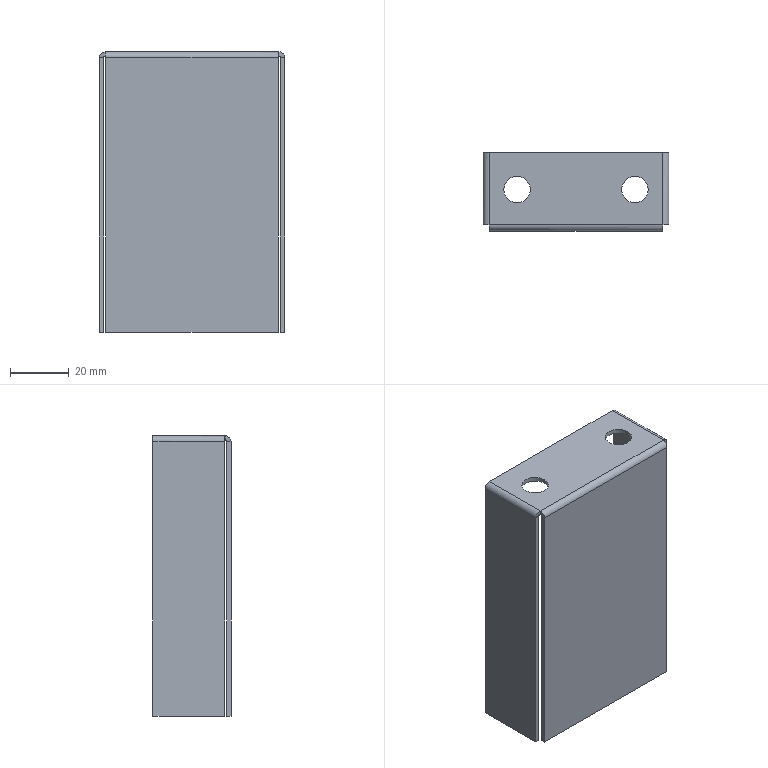Part | SolidWorks | features BaseBody 1 | 1 solid | 34 faces | box 63 x 26.5 x 95.1 mm | volume 17261 mm3 | plane 20 | cylinder 10 | spline 4 | commonest cylinder face diameters 9 x4 1 x3 4 x3
STEP:
#1=CARTESIAN_POINT('',(-24.5,0.,-1.5));
#2=VERTEX_POINT('',#1);
#3=CARTESIAN_POINT('',(-24.5,0.,0.));
#4=VERTEX_POINT('',#3);
#5=CARTESIAN_POINT('',(-24.5,0.,-1.5));
#6=DIRECTION('',(0.,0.,1.));
#7=VECTOR('',#6,1000.);
#8=LINE('',#5,#7);
#9=EDGE_CURVE('',#2,#4,#8,.T.);
#10=ORIENTED_EDGE('',*,*,#9,.F.);
#11=CARTESIAN_POINT('',(-15.5,0.,-1.5));
#12=VERTEX_POINT('',#11);
#13=CARTESIAN_POINT('',(-20.,0.,-1.5));
#14=DIRECTION('',(0.,0.,1.));
#15=DIRECTION('',(1.,0.,0.));
#16=AXIS2_PLACEMENT_3D('',#13,#14,#15);
#17=CIRCLE('',#16,4.5);
#18=EDGE_CURVE('',#12,#2,#17,.T.);
#19=ORIENTED_EDGE('',*,*,#18,.F.);
#20=CARTESIAN_POINT('',(-15.5,0.,0.));
#21=VERTEX_POINT('',#20);
#22=CARTESIAN_POINT('',(-15.5,0.,-1.5));
#23=DIRECTION('',(0.,0.,1.));
#24=VECTOR('',#23,1000.);
#25=LINE('',#22,#24);
#26=EDGE_CURVE('',#12,#21,#25,.T.);
#27=ORIENTED_EDGE('',*,*,#26,.T.);
#28=CARTESIAN_POINT('',(-20.,0.,0.));
#29=DIRECTION('',(0.,0.,1.));
#30=DIRECTION('',(1.,0.,0.));
#31=AXIS2_PLACEMENT_3D('',#28,#29,#30);
#32=CIRCLE('',#31,4.5);
#33=EDGE_CURVE('',#21,#4,#32,.T.);
#34=ORIENTED_EDGE('',*,*,#33,.T.);
#35=EDGE_LOOP('',(#10,#19,#27,#34));
#36=FACE_OUTER_BOUND('',#35,.T.);
#37=CARTESIAN_POINT('',(-20.,0.,-1.5));
#38=DIRECTION('',(0.,0.,1.));
#39=DIRECTION('',(1.,0.,0.));
#40=AXIS2_PLACEMENT_3D('',#37,#38,#39);
#41=CYLINDRICAL_SURFACE('',#40,4.5);
#42=ADVANCED_FACE('',(#36),#41,.F.);
#43=CARTESIAN_POINT('',(15.5,0.,-1.5));
#44=VERTEX_POINT('',#43);
#45=CARTESIAN_POINT('',(15.5,0.,0.));
#46=VERTEX_POINT('',#45);
#47=CARTESIAN_POINT('',(15.5,0.,-1.5));
#48=DIRECTION('',(0.,0.,1.));
#49=VECTOR('',#48,1000.);
#50=LINE('',#47,#49);
#51=EDGE_CURVE('',#44,#46,#50,.T.);
#52=ORIENTED_EDGE('',*,*,#51,.F.);
#53=CARTESIAN_POINT('',(24.5,0.,-1.5));
#54=VERTEX_POINT('',#53);
#55=CARTESIAN_POINT('',(20.,0.,-1.5));
#56=DIRECTION('',(0.,0.,1.));
#57=DIRECTION('',(-1.,0.,0.));
#58=AXIS2_PLACEMENT_3D('',#55,#56,#57);
#59=CIRCLE('',#58,4.5);
#60=EDGE_CURVE('',#54,#44,#59,.T.);
#61=ORIENTED_EDGE('',*,*,#60,.F.);
#62=CARTESIAN_POINT('',(24.5,0.,0.));
#63=VERTEX_POINT('',#62);
#64=CARTESIAN_POINT('',(24.5,0.,-1.5));
#65=DIRECTION('',(0.,0.,1.));
#66=VECTOR('',#65,1000.);
#67=LINE('',#64,#66);
#68=EDGE_CURVE('',#54,#63,#67,.T.);
#69=ORIENTED_EDGE('',*,*,#68,.T.);
#70=CARTESIAN_POINT('',(20.,0.,0.));
#71=DIRECTION('',(0.,0.,1.));
#72=DIRECTION('',(-1.,0.,0.));
#73=AXIS2_PLACEMENT_3D('',#70,#71,#72);
#74=CIRCLE('',#73,4.5);
#75=EDGE_CURVE('',#63,#46,#74,.T.);
#76=ORIENTED_EDGE('',*,*,#75,.T.);
#77=EDGE_LOOP('',(#52,#61,#69,#76));
#78=FACE_OUTER_BOUND('',#77,.T.);
#79=CARTESIAN_POINT('',(20.,0.,-1.5));
#80=DIRECTION('',(0.,0.,1.));
#81=DIRECTION('',(1.,0.,0.));
#82=AXIS2_PLACEMENT_3D('',#79,#80,#81);
#83=CYLINDRICAL_SURFACE('',#82,4.5);
#84=ADVANCED_FACE('',(#78),#83,.F.);
#85=CARTESIAN_POINT('',(31.5,-11.793,-95.1));
#86=VERTEX_POINT('',#85);
#87=CARTESIAN_POINT('',(30.,-11.793,-95.1));
#88=VERTEX_POINT('',#87);
#89=CARTESIAN_POINT('',(31.5,-11.793,-95.1));
#90=DIRECTION('',(-1.,0.,0.));
#91=VECTOR('',#90,1000.);
#92=LINE('',#89,#91);
#93=EDGE_CURVE('',#86,#88,#92,.T.);
#94=ORIENTED_EDGE('',*,*,#93,.F.);
#95=CARTESIAN_POINT('',(31.5,-11.793,-2.));
#96=VERTEX_POINT('',#95);
#97=CARTESIAN_POINT('',(31.5,-11.793,0.));
#98=DIRECTION('',(0.,0.,-1.));
#99=VECTOR('',#98,1000.);
#100=LINE('',#97,#99);
#101=EDGE_CURVE('',#96,#86,#100,.T.);
#102=ORIENTED_EDGE('',*,*,#101,.F.);
#103=CARTESIAN_POINT('',(30.,-11.793,-2.));
#104=VERTEX_POINT('',#103);
#105=CARTESIAN_POINT('',(30.,-11.793,-2.));
#106=DIRECTION('',(-1.,0.,0.));
#107=VECTOR('',#106,1000.);
#108=LINE('',#105,#107);
#109=EDGE_CURVE('',#96,#104,#108,.T.);
#110=ORIENTED_EDGE('',*,*,#109,.T.);
#111=CARTESIAN_POINT('',(30.,-11.793,-1.5));
#112=DIRECTION('',(0.,0.,-1.));
#113=VECTOR('',#112,1000.);
#114=LINE('',#111,#113);
#115=EDGE_CURVE('',#104,#88,#114,.T.);
#116=ORIENTED_EDGE('',*,*,#115,.T.);
#117=EDGE_LOOP('',(#94,#102,#110,#116));
#118=FACE_OUTER_BOUND('',#117,.T.);
#119=CARTESIAN_POINT('',(30.,-11.793,-1.5));
#120=DIRECTION('',(0.,1.,0.));
#121=DIRECTION('',(0.,0.,-1.));
#122=AXIS2_PLACEMENT_3D('',#119,#120,#121);
#123=PLANE('',#122);
#124=ADVANCED_FACE('',(#118),#123,.F.);
#125=CARTESIAN_POINT('',(31.5,12.5,-95.1));
#126=VERTEX_POINT('',#125);
#127=CARTESIAN_POINT('',(31.5,12.5,-95.1));
#128=DIRECTION('',(0.,1.,0.));
#129=VECTOR('',#128,1000.);
#130=LINE('',#127,#129);
#131=EDGE_CURVE('',#86,#126,#130,.T.);
#132=ORIENTED_EDGE('',*,*,#131,.F.);
#133=ORIENTED_EDGE('',*,*,#93,.T.);
#134=CARTESIAN_POINT('',(30.,12.5,-95.1));
#135=VERTEX_POINT('',#134);
#136=CARTESIAN_POINT('',(30.,12.5,-95.1));
#137=DIRECTION('',(0.,1.,0.));
#138=VECTOR('',#137,1000.);
#139=LINE('',#136,#138);
#140=EDGE_CURVE('',#88,#135,#139,.T.);
#141=ORIENTED_EDGE('',*,*,#140,.T.);
#142=CARTESIAN_POINT('',(31.5,12.5,-95.1));
#143=DIRECTION('',(-1.,0.,0.));
#144=VECTOR('',#143,1000.);
#145=LINE('',#142,#144);
#146=EDGE_CURVE('',#126,#135,#145,.T.);
#147=ORIENTED_EDGE('',*,*,#146,.F.);
#148=EDGE_LOOP('',(#132,#133,#141,#147));
#149=FACE_OUTER_BOUND('',#148,.T.);
#150=CARTESIAN_POINT('',(31.5,12.5,-95.1));
#151=DIRECTION('',(0.,0.,1.));
#152=DIRECTION('',(1.,0.,0.));
#153=AXIS2_PLACEMENT_3D('',#150,#151,#152);
#154=PLANE('',#153);
#155=ADVANCED_FACE('',(#149),#154,.F.);
#156=ORIENTED_EDGE('',*,*,#115,.F.);
#157=CARTESIAN_POINT('',(30.,12.5,-2.));
#158=VERTEX_POINT('',#157);
#159=CARTESIAN_POINT('',(30.,12.5,-2.));
#160=DIRECTION('',(0.,-1.,0.));
#161=VECTOR('',#160,1000.);
#162=LINE('',#159,#161);
#163=EDGE_CURVE('',#158,#104,#162,.T.);
#164=ORIENTED_EDGE('',*,*,#163,.F.);
#165=CARTESIAN_POINT('',(30.,12.5,-1.5));
#166=DIRECTION('',(0.,0.,1.));
#167=VECTOR('',#166,1000.);
#168=LINE('',#165,#167);
#169=EDGE_CURVE('',#135,#158,#168,.T.);
#170=ORIENTED_EDGE('',*,*,#169,.F.);
#171=ORIENTED_EDGE('',*,*,#140,.F.);
#172=EDGE_LOOP('',(#156,#164,#170,#171));
#173=FACE_OUTER_BOUND('',#172,.T.);
#174=CARTESIAN_POINT('',(30.,0.,0.));
#175=DIRECTION('',(-1.,0.,0.));
#176=DIRECTION('',(0.,0.,1.));
#177=AXIS2_PLACEMENT_3D('',#174,#175,#176);
#178=PLANE('',#177);
#179=ADVANCED_FACE('',(#173),#178,.T.);
#180=CARTESIAN_POINT('',(31.5,12.5,-2.));
#181=VERTEX_POINT('',#180);
#182=CARTESIAN_POINT('',(31.5,0.,-2.));
#183=DIRECTION('',(0.,1.,0.));
#184=VECTOR('',#183,1000.);
#185=LINE('',#182,#184);
#186=EDGE_CURVE('',#96,#181,#185,.T.);
#187=ORIENTED_EDGE('',*,*,#186,.F.);
#188=ORIENTED_EDGE('',*,*,#101,.T.);
#189=ORIENTED_EDGE('',*,*,#131,.T.);
#190=CARTESIAN_POINT('',(31.5,12.5,-1.5));
#191=DIRECTION('',(0.,0.,1.));
#192=VECTOR('',#191,1000.);
#193=LINE('',#190,#192);
#194=EDGE_CURVE('',#126,#181,#193,.T.);
#195=ORIENTED_EDGE('',*,*,#194,.T.);
#196=EDGE_LOOP('',(#187,#188,#189,#195));
#197=FACE_OUTER_BOUND('',#196,.T.);
#198=CARTESIAN_POINT('',(31.5,0.,0.));
#199=DIRECTION('',(-1.,0.,0.));
#200=DIRECTION('',(0.,0.,1.));
#201=AXIS2_PLACEMENT_3D('',#198,#199,#200);
#202=PLANE('',#201);
#203=ADVANCED_FACE('',(#197),#202,.F.);
#204=CARTESIAN_POINT('',(30.,12.5,-2.));
#205=DIRECTION('',(1.,0.,0.));
#206=VECTOR('',#205,1000.);
#207=LINE('',#204,#206);
#208=EDGE_CURVE('',#158,#181,#207,.T.);
#209=ORIENTED_EDGE('',*,*,#208,.T.);
#210=ORIENTED_EDGE('',*,*,#194,.F.);
#211=ORIENTED_EDGE('',*,*,#146,.T.);
#212=ORIENTED_EDGE('',*,*,#169,.T.);
#213=EDGE_LOOP('',(#209,#210,#211,#212));
#214=FACE_OUTER_BOUND('',#213,.T.);
#215=CARTESIAN_POINT('',(31.5,12.5,-1.5));
#216=DIRECTION('',(0.,-1.,0.));
#217=DIRECTION('',(-1.,0.,0.));
#218=AXIS2_PLACEMENT_3D('',#215,#216,#217);
#219=PLANE('',#218);
#220=ADVANCED_FACE('',(#214),#219,.F.);
#221=CARTESIAN_POINT('',(29.5,-12.,-1.5));
#222=VERTEX_POINT('',#221);
#223=CARTESIAN_POINT('',(29.5,12.5,-1.5));
#224=VERTEX_POINT('',#223);
#225=CARTESIAN_POINT('',(29.5,-12.,-1.5));
#226=DIRECTION('',(0.,1.,0.));
#227=VECTOR('',#226,1000.);
#228=LINE('',#225,#227);
#229=EDGE_CURVE('',#222,#224,#228,.T.);
#230=ORIENTED_EDGE('',*,*,#229,.T.);
#231=CARTESIAN_POINT('',(29.5,12.5,-2.));
#232=DIRECTION('',(0.,1.,0.));
#233=DIRECTION('',(0.,0.,-1.));
#234=AXIS2_PLACEMENT_3D('',#231,#232,#233);
#235=CIRCLE('',#234,0.5);
#236=EDGE_CURVE('',#224,#158,#235,.T.);
#237=ORIENTED_EDGE('',*,*,#236,.T.);
#238=ORIENTED_EDGE('',*,*,#163,.T.);
#239=CARTESIAN_POINT('',(30.,-11.793,-2.));
#240=CARTESIAN_POINT('',(30.,-11.827,-1.869));
#241=CARTESIAN_POINT('',(29.946,-11.862,-1.739));
#242=CARTESIAN_POINT('',(29.761,-11.931,-1.554));
#243=CARTESIAN_POINT('',(29.631,-11.965,-1.5));
#244=CARTESIAN_POINT('',(29.5,-12.,-1.5));
#245=B_SPLINE_CURVE_WITH_KNOTS('',3,(#239,#240,#241,#242,#243,#244),.UNSPECIFIED.,.F.,.F.,(4,2,4),(0.,0.5,1.),.UNSPECIFIED.);
#246=EDGE_CURVE('',#104,#222,#245,.T.);
#247=ORIENTED_EDGE('',*,*,#246,.T.);
#248=EDGE_LOOP('',(#230,#237,#238,#247));
#249=FACE_OUTER_BOUND('',#248,.T.);
#250=CARTESIAN_POINT('',(29.5,-12.,-2.));
#251=DIRECTION('',(0.,-1.,0.));
#252=DIRECTION('',(1.,0.,0.));
#253=AXIS2_PLACEMENT_3D('',#250,#251,#252);
#254=CYLINDRICAL_SURFACE('',#253,0.5);
#255=ADVANCED_FACE('',(#249),#254,.F.);
#256=CARTESIAN_POINT('',(29.5,-12.,0.));
#257=VERTEX_POINT('',#256);
#258=CARTESIAN_POINT('',(29.5,12.5,0.));
#259=VERTEX_POINT('',#258);
#260=CARTESIAN_POINT('',(29.5,-12.,0.));
#261=DIRECTION('',(0.,1.,0.));
#262=VECTOR('',#261,1000.);
#263=LINE('',#260,#262);
#264=EDGE_CURVE('',#257,#259,#263,.T.);
#265=ORIENTED_EDGE('',*,*,#264,.F.);
#266=CARTESIAN_POINT('',(31.5,-11.793,-2.));
#267=CARTESIAN_POINT('',(31.5,-11.81,-1.738));
#268=CARTESIAN_POINT('',(31.448,-11.827,-1.477));
#269=CARTESIAN_POINT('',(31.248,-11.862,-0.9928));
#270=CARTESIAN_POINT('',(31.099,-11.879,-0.7709));
#271=CARTESIAN_POINT('',(30.729,-11.914,-0.4007));
#272=CARTESIAN_POINT('',(30.507,-11.931,-0.2524));
#273=CARTESIAN_POINT('',(30.023,-11.965,-0.05205));
#274=CARTESIAN_POINT('',(29.762,-11.983,0.));
#275=CARTESIAN_POINT('',(29.5,-12.,0.));
#276=B_SPLINE_CURVE_WITH_KNOTS('',3,(#266,#267,#268,#269,#270,#271,#272,#273,#274,#275),.UNSPECIFIED.,.F.,.F.,(4,2,2,2,4),(0.,0.25,0.5,0.75,1.),.UNSPECIFIED.);
#277=EDGE_CURVE('',#96,#257,#276,.T.);
#278=ORIENTED_EDGE('',*,*,#277,.F.);
#279=ORIENTED_EDGE('',*,*,#186,.T.);
#280=CARTESIAN_POINT('',(29.5,12.5,-2.));
#281=DIRECTION('',(0.,1.,0.));
#282=DIRECTION('',(0.,0.,-1.));
#283=AXIS2_PLACEMENT_3D('',#280,#281,#282);
#284=CIRCLE('',#283,2.);
#285=EDGE_CURVE('',#259,#181,#284,.T.);
#286=ORIENTED_EDGE('',*,*,#285,.F.);
#287=EDGE_LOOP('',(#265,#278,#279,#286));
#288=FACE_OUTER_BOUND('',#287,.T.);
#289=CARTESIAN_POINT('',(29.5,-12.,-2.));
#290=DIRECTION('',(0.,-1.,0.));
#291=DIRECTION('',(1.,0.,0.));
#292=AXIS2_PLACEMENT_3D('',#289,#290,#291);
#293=CYLINDRICAL_SURFACE('',#292,2.);
#294=ADVANCED_FACE('',(#288),#293,.T.);
#295=ORIENTED_EDGE('',*,*,#246,.F.);
#296=ORIENTED_EDGE('',*,*,#109,.F.);
#297=ORIENTED_EDGE('',*,*,#277,.T.);
#298=CARTESIAN_POINT('',(29.5,-12.,-1.5));
#299=DIRECTION('',(0.,0.,1.));
#300=VECTOR('',#299,1000.);
#301=LINE('',#298,#300);
#302=EDGE_CURVE('',#222,#257,#301,.T.);
#303=ORIENTED_EDGE('',*,*,#302,.F.);
#304=EDGE_LOOP('',(#295,#296,#297,#303));
#305=FACE_OUTER_BOUND('',#304,.T.);
#306=CARTESIAN_POINT('',(31.515,-11.793,-2.));
#307=CARTESIAN_POINT('',(31.515,-11.81,-1.736));
#308=CARTESIAN_POINT('',(31.463,-11.827,-1.473));
#309=CARTESIAN_POINT('',(31.261,-11.862,-0.9852));
#310=CARTESIAN_POINT('',(31.111,-11.879,-0.7617));
#311=CARTESIAN_POINT('',(30.738,-11.914,-0.3887));
#312=CARTESIAN_POINT('',(30.515,-11.931,-0.2393));
#313=CARTESIAN_POINT('',(30.027,-11.965,-0.03745));
#314=CARTESIAN_POINT('',(29.764,-11.983,0.015));
#315=CARTESIAN_POINT('',(29.5,-12.,0.015));
#316=CARTESIAN_POINT('',(31.5,-11.793,-2.));
#317=CARTESIAN_POINT('',(31.5,-11.81,-1.738));
#318=CARTESIAN_POINT('',(31.448,-11.827,-1.477));
#319=CARTESIAN_POINT('',(31.248,-11.862,-0.9928));
#320=CARTESIAN_POINT('',(31.099,-11.879,-0.7709));
#321=CARTESIAN_POINT('',(30.729,-11.914,-0.4007));
#322=CARTESIAN_POINT('',(30.507,-11.931,-0.2524));
#323=CARTESIAN_POINT('',(30.023,-11.965,-0.05205));
#324=CARTESIAN_POINT('',(29.762,-11.983,0.));
#325=CARTESIAN_POINT('',(29.5,-12.,0.));
#326=CARTESIAN_POINT('',(30.,-11.793,-2.));
#327=CARTESIAN_POINT('',(30.,-11.81,-1.935));
#328=CARTESIAN_POINT('',(29.987,-11.827,-1.869));
#329=CARTESIAN_POINT('',(29.937,-11.862,-1.748));
#330=CARTESIAN_POINT('',(29.9,-11.879,-1.693));
#331=CARTESIAN_POINT('',(29.807,-11.914,-1.6));
#332=CARTESIAN_POINT('',(29.752,-11.931,-1.563));
#333=CARTESIAN_POINT('',(29.631,-11.965,-1.513));
#334=CARTESIAN_POINT('',(29.565,-11.983,-1.5));
#335=CARTESIAN_POINT('',(29.5,-12.,-1.5));
#336=CARTESIAN_POINT('',(29.985,-11.793,-2.));
#337=CARTESIAN_POINT('',(29.985,-11.81,-1.937));
#338=CARTESIAN_POINT('',(29.972,-11.827,-1.873));
#339=CARTESIAN_POINT('',(29.924,-11.862,-1.756));
#340=CARTESIAN_POINT('',(29.888,-11.879,-1.702));
#341=CARTESIAN_POINT('',(29.798,-11.914,-1.612));
#342=CARTESIAN_POINT('',(29.744,-11.931,-1.576));
#343=CARTESIAN_POINT('',(29.627,-11.965,-1.528));
#344=CARTESIAN_POINT('',(29.563,-11.983,-1.515));
#345=CARTESIAN_POINT('',(29.5,-12.,-1.515));
#346=B_SPLINE_SURFACE_WITH_KNOTS('',1,3,((#306,#307,#308,#309,#310,#311,#312,#313,#314,#315),(#316,#317,#318,#319,#320,#321,#322,#323,#324,#325),(#326,#327,#328,#329,#330,#331,#332,#333,#334,#335),(#336,#337,#338,#339,#340,#341,#342,#343,#344,#345)),.UNSPECIFIED.,.F.,.F.,.F.,(2,1,1,2),(4,2,2,2,4),(-0.01,0.,1.,1.01),(0.,0.25,0.5,0.75,1.),.UNSPECIFIED.);
#347=ADVANCED_FACE('',(#305),#346,.F.);
#348=ORIENTED_EDGE('',*,*,#208,.F.);
#349=ORIENTED_EDGE('',*,*,#236,.F.);
#350=CARTESIAN_POINT('',(29.5,12.5,-1.5));
#351=DIRECTION('',(0.,0.,1.));
#352=VECTOR('',#351,1000.);
#353=LINE('',#350,#352);
#354=EDGE_CURVE('',#224,#259,#353,.T.);
#355=ORIENTED_EDGE('',*,*,#354,.T.);
#356=ORIENTED_EDGE('',*,*,#285,.T.);
#357=EDGE_LOOP('',(#348,#349,#355,#356));
#358=FACE_OUTER_BOUND('',#357,.T.);
#359=CARTESIAN_POINT('',(29.5,12.5,-2.));
#360=DIRECTION('',(0.,1.,0.));
#361=DIRECTION('',(1.,0.,0.));
#362=AXIS2_PLACEMENT_3D('',#359,#360,#361);
#363=PLANE('',#362);
#364=ADVANCED_FACE('',(#358),#363,.T.);
#365=CARTESIAN_POINT('',(-29.293,-14.,-95.1));
#366=VERTEX_POINT('',#365);
#367=CARTESIAN_POINT('',(-29.293,-12.5,-95.1));
#368=VERTEX_POINT('',#367);
#369=CARTESIAN_POINT('',(-29.293,-14.,-95.1));
#370=DIRECTION('',(0.,1.,0.));
#371=VECTOR('',#370,1000.);
#372=LINE('',#369,#371);
#373=EDGE_CURVE('',#366,#368,#372,.T.);
#374=ORIENTED_EDGE('',*,*,#373,.F.);
#375=CARTESIAN_POINT('',(-29.293,-14.,-2.));
#376=VERTEX_POINT('',#375);
#377=CARTESIAN_POINT('',(-29.293,-14.,0.));
#378=DIRECTION('',(0.,0.,-1.));
#379=VECTOR('',#378,1000.);
#380=LINE('',#377,#379);
#381=EDGE_CURVE('',#376,#366,#380,.T.);
#382=ORIENTED_EDGE('',*,*,#381,.F.);
#383=CARTESIAN_POINT('',(-29.293,-12.5,-2.));
#384=VERTEX_POINT('',#383);
#385=CARTESIAN_POINT('',(-29.293,-12.5,-2.));
#386=DIRECTION('',(0.,1.,0.));
#387=VECTOR('',#386,1000.);
#388=LINE('',#385,#387);
#389=EDGE_CURVE('',#376,#384,#388,.T.);
#390=ORIENTED_EDGE('',*,*,#389,.T.);
#391=CARTESIAN_POINT('',(-29.293,-12.5,-1.5));
#392=DIRECTION('',(0.,0.,-1.));
#393=VECTOR('',#392,1000.);
#394=LINE('',#391,#393);
#395=EDGE_CURVE('',#384,#368,#394,.T.);
#396=ORIENTED_EDGE('',*,*,#395,.T.);
#397=EDGE_LOOP('',(#374,#382,#390,#396));
#398=FACE_OUTER_BOUND('',#397,.T.);
#399=CARTESIAN_POINT('',(-29.293,-12.5,-1.5));
#400=DIRECTION('',(1.,0.,0.));
#401=DIRECTION('',(0.,1.,0.));
#402=AXIS2_PLACEMENT_3D('',#399,#400,#401);
#403=PLANE('',#402);
#404=ADVANCED_FACE('',(#398),#403,.F.);
#405=CARTESIAN_POINT('',(29.293,-14.,-95.1));
#406=VERTEX_POINT('',#405);
#407=CARTESIAN_POINT('',(29.293,-12.5,-95.1));
#408=VERTEX_POINT('',#407);
#409=CARTESIAN_POINT('',(29.293,-14.,-95.1));
#410=DIRECTION('',(0.,1.,0.));
#411=VECTOR('',#410,1000.);
#412=LINE('',#409,#411);
#413=EDGE_CURVE('',#406,#408,#412,.T.);
#414=ORIENTED_EDGE('',*,*,#413,.F.);
#415=CARTESIAN_POINT('',(30.,-14.,-95.1));
#416=DIRECTION('',(1.,0.,0.));
#417=VECTOR('',#416,1000.);
#418=LINE('',#415,#417);
#419=EDGE_CURVE('',#366,#406,#418,.T.);
#420=ORIENTED_EDGE('',*,*,#419,.F.);
#421=ORIENTED_EDGE('',*,*,#373,.T.);
#422=CARTESIAN_POINT('',(30.,-12.5,-95.1));
#423=DIRECTION('',(1.,0.,0.));
#424=VECTOR('',#423,1000.);
#425=LINE('',#422,#424);
#426=EDGE_CURVE('',#368,#408,#425,.T.);
#427=ORIENTED_EDGE('',*,*,#426,.T.);
#428=EDGE_LOOP('',(#414,#420,#421,#427));
#429=FACE_OUTER_BOUND('',#428,.T.);
#430=CARTESIAN_POINT('',(30.,-14.,-95.1));
#431=DIRECTION('',(0.,0.,1.));
#432=DIRECTION('',(0.,-1.,0.));
#433=AXIS2_PLACEMENT_3D('',#430,#431,#432);
#434=PLANE('',#433);
#435=ADVANCED_FACE('',(#429),#434,.F.);
#436=CARTESIAN_POINT('',(29.293,-12.5,-2.));
#437=VERTEX_POINT('',#436);
#438=CARTESIAN_POINT('',(30.,-12.5,-2.));
#439=DIRECTION('',(-1.,0.,0.));
#440=VECTOR('',#439,1000.);
#441=LINE('',#438,#440);
#442=EDGE_CURVE('',#437,#384,#441,.T.);
#443=ORIENTED_EDGE('',*,*,#442,.F.);
#444=CARTESIAN_POINT('',(29.293,-12.5,-1.5));
#445=DIRECTION('',(0.,0.,-1.));
#446=VECTOR('',#445,1000.);
#447=LINE('',#444,#446);
#448=EDGE_CURVE('',#437,#408,#447,.T.);
#449=ORIENTED_EDGE('',*,*,#448,.T.);
#450=ORIENTED_EDGE('',*,*,#426,.F.);
#451=ORIENTED_EDGE('',*,*,#395,.F.);
#452=EDGE_LOOP('',(#443,#449,#450,#451));
#453=FACE_OUTER_BOUND('',#452,.T.);
#454=CARTESIAN_POINT('',(0.,-12.5,0.));
#455=DIRECTION('',(0.,1.,0.));
#456=DIRECTION('',(0.,0.,-1.));
#457=AXIS2_PLACEMENT_3D('',#454,#455,#456);
#458=PLANE('',#457);
#459=ADVANCED_FACE('',(#453),#458,.T.);
#460=CARTESIAN_POINT('',(29.293,-14.,-2.));
#461=VERTEX_POINT('',#460);
#462=CARTESIAN_POINT('',(29.293,-14.,0.));
#463=DIRECTION('',(0.,0.,-1.));
#464=VECTOR('',#463,1000.);
#465=LINE('',#462,#464);
#466=EDGE_CURVE('',#461,#406,#465,.T.);
#467=ORIENTED_EDGE('',*,*,#466,.F.);
#468=CARTESIAN_POINT('',(0.,-14.,-2.));
#469=DIRECTION('',(1.,0.,0.));
#470=VECTOR('',#469,1000.);
#471=LINE('',#468,#470);
#472=EDGE_CURVE('',#376,#461,#471,.T.);
#473=ORIENTED_EDGE('',*,*,#472,.F.);
#474=ORIENTED_EDGE('',*,*,#381,.T.);
#475=ORIENTED_EDGE('',*,*,#419,.T.);
#476=EDGE_LOOP('',(#467,#473,#474,#475));
#477=FACE_OUTER_BOUND('',#476,.T.);
#478=CARTESIAN_POINT('',(0.,-14.,0.));
#479=DIRECTION('',(0.,1.,0.));
#480=DIRECTION('',(0.,0.,-1.));
#481=AXIS2_PLACEMENT_3D('',#478,#479,#480);
#482=PLANE('',#481);
#483=ADVANCED_FACE('',(#477),#482,.F.);
#484=ORIENTED_EDGE('',*,*,#466,.T.);
#485=ORIENTED_EDGE('',*,*,#413,.T.);
#486=ORIENTED_EDGE('',*,*,#448,.F.);
#487=CARTESIAN_POINT('',(29.293,-12.5,-2.));
#488=DIRECTION('',(0.,1.,0.));
#489=VECTOR('',#488,1000.);
#490=LINE('',#487,#489);
#491=EDGE_CURVE('',#461,#437,#490,.T.);
#492=ORIENTED_EDGE('',*,*,#491,.F.);
#493=EDGE_LOOP('',(#484,#485,#486,#492));
#494=FACE_OUTER_BOUND('',#493,.T.);
#495=CARTESIAN_POINT('',(29.293,-12.5,-1.5));
#496=DIRECTION('',(1.,0.,0.));
#497=DIRECTION('',(0.,1.,0.));
#498=AXIS2_PLACEMENT_3D('',#495,#496,#497);
#499=PLANE('',#498);
#500=ADVANCED_FACE('',(#494),#499,.T.);
#501=CARTESIAN_POINT('',(-29.5,-12.,-1.5));
#502=VERTEX_POINT('',#501);
#503=CARTESIAN_POINT('',(-29.5,-12.,-1.5));
#504=DIRECTION('',(1.,0.,0.));
#505=VECTOR('',#504,1000.);
#506=LINE('',#503,#505);
#507=EDGE_CURVE('',#502,#222,#506,.T.);
#508=ORIENTED_EDGE('',*,*,#507,.T.);
#509=CARTESIAN_POINT('',(29.5,-12.,-1.5));
#510=CARTESIAN_POINT('',(29.465,-12.131,-1.5));
#511=CARTESIAN_POINT('',(29.431,-12.261,-1.554));
#512=CARTESIAN_POINT('',(29.362,-12.446,-1.739));
#513=CARTESIAN_POINT('',(29.327,-12.5,-1.869));
#514=CARTESIAN_POINT('',(29.293,-12.5,-2.));
#515=B_SPLINE_CURVE_WITH_KNOTS('',3,(#509,#510,#511,#512,#513,#514),.UNSPECIFIED.,.F.,.F.,(4,2,4),(0.,0.5,1.),.UNSPECIFIED.);
#516=EDGE_CURVE('',#222,#437,#515,.T.);
#517=ORIENTED_EDGE('',*,*,#516,.T.);
#518=ORIENTED_EDGE('',*,*,#442,.T.);
#519=CARTESIAN_POINT('',(-29.293,-12.5,-2.));
#520=CARTESIAN_POINT('',(-29.327,-12.5,-1.869));
#521=CARTESIAN_POINT('',(-29.362,-12.446,-1.739));
#522=CARTESIAN_POINT('',(-29.431,-12.261,-1.554));
#523=CARTESIAN_POINT('',(-29.465,-12.131,-1.5));
#524=CARTESIAN_POINT('',(-29.5,-12.,-1.5));
#525=B_SPLINE_CURVE_WITH_KNOTS('',3,(#519,#520,#521,#522,#523,#524),.UNSPECIFIED.,.F.,.F.,(4,2,4),(0.,0.5,1.),.UNSPECIFIED.);
#526=EDGE_CURVE('',#384,#502,#525,.T.);
#527=ORIENTED_EDGE('',*,*,#526,.T.);
#528=EDGE_LOOP('',(#508,#517,#518,#527));
#529=FACE_OUTER_BOUND('',#528,.T.);
#530=CARTESIAN_POINT('',(-29.5,-12.,-2.));
#531=DIRECTION('',(-1.,0.,0.));
#532=DIRECTION('',(0.,-1.,0.));
#533=AXIS2_PLACEMENT_3D('',#530,#531,#532);
#534=CYLINDRICAL_SURFACE('',#533,0.5);
#535=ADVANCED_FACE('',(#529),#534,.F.);
#536=CARTESIAN_POINT('',(-29.5,-12.,0.));
#537=VERTEX_POINT('',#536);
#538=CARTESIAN_POINT('',(-29.5,-12.,0.));
#539=DIRECTION('',(1.,0.,0.));
#540=VECTOR('',#539,1000.);
#541=LINE('',#538,#540);
#542=EDGE_CURVE('',#537,#257,#541,.T.);
#543=ORIENTED_EDGE('',*,*,#542,.F.);
#544=CARTESIAN_POINT('',(-29.293,-14.,-2.));
#545=CARTESIAN_POINT('',(-29.31,-14.,-1.738));
#546=CARTESIAN_POINT('',(-29.327,-13.948,-1.477));
#547=CARTESIAN_POINT('',(-29.362,-13.748,-0.9928));
#548=CARTESIAN_POINT('',(-29.379,-13.599,-0.7709));
#549=CARTESIAN_POINT('',(-29.414,-13.229,-0.4007));
#550=CARTESIAN_POINT('',(-29.431,-13.007,-0.2524));
#551=CARTESIAN_POINT('',(-29.465,-12.523,-0.05205));
#552=CARTESIAN_POINT('',(-29.483,-12.262,0.));
#553=CARTESIAN_POINT('',(-29.5,-12.,0.));
#554=B_SPLINE_CURVE_WITH_KNOTS('',3,(#544,#545,#546,#547,#548,#549,#550,#551,#552,#553),.UNSPECIFIED.,.F.,.F.,(4,2,2,2,4),(0.,0.25,0.5,0.75,1.),.UNSPECIFIED.);
#555=EDGE_CURVE('',#376,#537,#554,.T.);
#556=ORIENTED_EDGE('',*,*,#555,.F.);
#557=ORIENTED_EDGE('',*,*,#472,.T.);
#558=CARTESIAN_POINT('',(29.5,-12.,0.));
#559=CARTESIAN_POINT('',(29.483,-12.262,0.));
#560=CARTESIAN_POINT('',(29.465,-12.523,-0.05205));
#561=CARTESIAN_POINT('',(29.431,-13.007,-0.2524));
#562=CARTESIAN_POINT('',(29.414,-13.229,-0.4007));
#563=CARTESIAN_POINT('',(29.379,-13.599,-0.7709));
#564=CARTESIAN_POINT('',(29.362,-13.748,-0.9928));
#565=CARTESIAN_POINT('',(29.327,-13.948,-1.477));
#566=CARTESIAN_POINT('',(29.31,-14.,-1.738));
#567=CARTESIAN_POINT('',(29.293,-14.,-2.));
#568=B_SPLINE_CURVE_WITH_KNOTS('',3,(#558,#559,#560,#561,#562,#563,#564,#565,#566,#567),.UNSPECIFIED.,.F.,.F.,(4,2,2,2,4),(0.,0.25,0.5,0.75,1.),.UNSPECIFIED.);
#569=EDGE_CURVE('',#257,#461,#568,.T.);
#570=ORIENTED_EDGE('',*,*,#569,.F.);
#571=EDGE_LOOP('',(#543,#556,#557,#570));
#572=FACE_OUTER_BOUND('',#571,.T.);
#573=CARTESIAN_POINT('',(-29.5,-12.,-2.));
#574=DIRECTION('',(-1.,0.,0.));
#575=DIRECTION('',(0.,-1.,0.));
#576=AXIS2_PLACEMENT_3D('',#573,#574,#575);
#577=CYLINDRICAL_SURFACE('',#576,2.);
#578=ADVANCED_FACE('',(#572),#577,.T.);
#579=ORIENTED_EDGE('',*,*,#526,.F.);
#580=ORIENTED_EDGE('',*,*,#389,.F.);
#581=ORIENTED_EDGE('',*,*,#555,.T.);
#582=CARTESIAN_POINT('',(-29.5,-12.,-1.5));
#583=DIRECTION('',(0.,0.,1.));
#584=VECTOR('',#583,1000.);
#585=LINE('',#582,#584);
#586=EDGE_CURVE('',#502,#537,#585,.T.);
#587=ORIENTED_EDGE('',*,*,#586,.F.);
#588=EDGE_LOOP('',(#579,#580,#581,#587));
#589=FACE_OUTER_BOUND('',#588,.T.);
#590=CARTESIAN_POINT('',(-29.293,-14.015,-2.));
#591=CARTESIAN_POINT('',(-29.31,-14.015,-1.736));
#592=CARTESIAN_POINT('',(-29.327,-13.963,-1.473));
#593=CARTESIAN_POINT('',(-29.362,-13.761,-0.9852));
#594=CARTESIAN_POINT('',(-29.379,-13.611,-0.7617));
#595=CARTESIAN_POINT('',(-29.414,-13.238,-0.3887));
#596=CARTESIAN_POINT('',(-29.431,-13.015,-0.2393));
#597=CARTESIAN_POINT('',(-29.465,-12.527,-0.03745));
#598=CARTESIAN_POINT('',(-29.483,-12.264,0.015));
#599=CARTESIAN_POINT('',(-29.5,-12.,0.015));
#600=CARTESIAN_POINT('',(-29.293,-14.,-2.));
#601=CARTESIAN_POINT('',(-29.31,-14.,-1.738));
#602=CARTESIAN_POINT('',(-29.327,-13.948,-1.477));
#603=CARTESIAN_POINT('',(-29.362,-13.748,-0.9928));
#604=CARTESIAN_POINT('',(-29.379,-13.599,-0.7709));
#605=CARTESIAN_POINT('',(-29.414,-13.229,-0.4007));
#606=CARTESIAN_POINT('',(-29.431,-13.007,-0.2524));
#607=CARTESIAN_POINT('',(-29.465,-12.523,-0.05205));
#608=CARTESIAN_POINT('',(-29.483,-12.262,0.));
#609=CARTESIAN_POINT('',(-29.5,-12.,0.));
#610=CARTESIAN_POINT('',(-29.293,-12.5,-2.));
#611=CARTESIAN_POINT('',(-29.31,-12.5,-1.935));
#612=CARTESIAN_POINT('',(-29.327,-12.487,-1.869));
#613=CARTESIAN_POINT('',(-29.362,-12.437,-1.748));
#614=CARTESIAN_POINT('',(-29.379,-12.4,-1.693));
#615=CARTESIAN_POINT('',(-29.414,-12.307,-1.6));
#616=CARTESIAN_POINT('',(-29.431,-12.252,-1.563));
#617=CARTESIAN_POINT('',(-29.465,-12.131,-1.513));
#618=CARTESIAN_POINT('',(-29.483,-12.065,-1.5));
#619=CARTESIAN_POINT('',(-29.5,-12.,-1.5));
#620=CARTESIAN_POINT('',(-29.293,-12.485,-2.));
#621=CARTESIAN_POINT('',(-29.31,-12.485,-1.937));
#622=CARTESIAN_POINT('',(-29.327,-12.472,-1.873));
#623=CARTESIAN_POINT('',(-29.362,-12.424,-1.756));
#624=CARTESIAN_POINT('',(-29.379,-12.388,-1.702));
#625=CARTESIAN_POINT('',(-29.414,-12.298,-1.612));
#626=CARTESIAN_POINT('',(-29.431,-12.244,-1.576));
#627=CARTESIAN_POINT('',(-29.465,-12.127,-1.528));
#628=CARTESIAN_POINT('',(-29.483,-12.063,-1.515));
#629=CARTESIAN_POINT('',(-29.5,-12.,-1.515));
#630=B_SPLINE_SURFACE_WITH_KNOTS('',1,3,((#590,#591,#592,#593,#594,#595,#596,#597,#598,#599),(#600,#601,#602,#603,#604,#605,#606,#607,#608,#609),(#610,#611,#612,#613,#614,#615,#616,#617,#618,#619),(#620,#621,#622,#623,#624,#625,#626,#627,#628,#629)),.UNSPECIFIED.,.F.,.F.,.F.,(2,1,1,2),(4,2,2,2,4),(-0.01,0.,1.,1.01),(0.,0.25,0.5,0.75,1.),.UNSPECIFIED.);
#631=ADVANCED_FACE('',(#589),#630,.F.);
#632=ORIENTED_EDGE('',*,*,#491,.T.);
#633=ORIENTED_EDGE('',*,*,#516,.F.);
#634=ORIENTED_EDGE('',*,*,#302,.T.);
#635=ORIENTED_EDGE('',*,*,#569,.T.);
#636=EDGE_LOOP('',(#632,#633,#634,#635));
#637=FACE_OUTER_BOUND('',#636,.T.);
#638=CARTESIAN_POINT('',(29.5,-12.,0.015));
#639=CARTESIAN_POINT('',(29.483,-12.264,0.015));
#640=CARTESIAN_POINT('',(29.465,-12.527,-0.03745));
#641=CARTESIAN_POINT('',(29.431,-13.015,-0.2393));
#642=CARTESIAN_POINT('',(29.414,-13.238,-0.3887));
#643=CARTESIAN_POINT('',(29.379,-13.611,-0.7617));
#644=CARTESIAN_POINT('',(29.362,-13.761,-0.9852));
#645=CARTESIAN_POINT('',(29.327,-13.963,-1.473));
#646=CARTESIAN_POINT('',(29.31,-14.015,-1.736));
#647=CARTESIAN_POINT('',(29.293,-14.015,-2.));
#648=CARTESIAN_POINT('',(29.5,-12.,0.));
#649=CARTESIAN_POINT('',(29.483,-12.262,0.));
#650=CARTESIAN_POINT('',(29.465,-12.523,-0.05205));
#651=CARTESIAN_POINT('',(29.431,-13.007,-0.2524));
#652=CARTESIAN_POINT('',(29.414,-13.229,-0.4007));
#653=CARTESIAN_POINT('',(29.379,-13.599,-0.7709));
#654=CARTESIAN_POINT('',(29.362,-13.748,-0.9928));
#655=CARTESIAN_POINT('',(29.327,-13.948,-1.477));
#656=CARTESIAN_POINT('',(29.31,-14.,-1.738));
#657=CARTESIAN_POINT('',(29.293,-14.,-2.));
#658=CARTESIAN_POINT('',(29.5,-12.,-1.5));
#659=CARTESIAN_POINT('',(29.483,-12.065,-1.5));
#660=CARTESIAN_POINT('',(29.465,-12.131,-1.513));
#661=CARTESIAN_POINT('',(29.431,-12.252,-1.563));
#662=CARTESIAN_POINT('',(29.414,-12.307,-1.6));
#663=CARTESIAN_POINT('',(29.379,-12.4,-1.693));
#664=CARTESIAN_POINT('',(29.362,-12.437,-1.748));
#665=CARTESIAN_POINT('',(29.327,-12.487,-1.869));
#666=CARTESIAN_POINT('',(29.31,-12.5,-1.935));
#667=CARTESIAN_POINT('',(29.293,-12.5,-2.));
#668=CARTESIAN_POINT('',(29.5,-12.,-1.515));
#669=CARTESIAN_POINT('',(29.483,-12.063,-1.515));
#670=CARTESIAN_POINT('',(29.465,-12.127,-1.528));
#671=CARTESIAN_POINT('',(29.431,-12.244,-1.576));
#672=CARTESIAN_POINT('',(29.414,-12.298,-1.612));
#673=CARTESIAN_POINT('',(29.379,-12.388,-1.702));
#674=CARTESIAN_POINT('',(29.362,-12.424,-1.756));
#675=CARTESIAN_POINT('',(29.327,-12.472,-1.873));
#676=CARTESIAN_POINT('',(29.31,-12.485,-1.937));
#677=CARTESIAN_POINT('',(29.293,-12.485,-2.));
#678=B_SPLINE_SURFACE_WITH_KNOTS('',1,3,((#638,#639,#640,#641,#642,#643,#644,#645,#646,#647),(#648,#649,#650,#651,#652,#653,#654,#655,#656,#657),(#658,#659,#660,#661,#662,#663,#664,#665,#666,#667),(#668,#669,#670,#671,#672,#673,#674,#675,#676,#677)),.UNSPECIFIED.,.F.,.F.,.F.,(2,1,1,2),(4,2,2,2,4),(-0.01,0.,1.,1.01),(0.,0.25,0.5,0.75,1.),.UNSPECIFIED.);
#679=ADVANCED_FACE('',(#637),#678,.F.);
#680=CARTESIAN_POINT('',(-30.,12.5,-2.));
#681=VERTEX_POINT('',#680);
#682=CARTESIAN_POINT('',(-31.5,12.5,-2.));
#683=VERTEX_POINT('',#682);
#684=CARTESIAN_POINT('',(-30.,12.5,-2.));
#685=DIRECTION('',(-1.,0.,0.));
#686=VECTOR('',#685,1000.);
#687=LINE('',#684,#686);
#688=EDGE_CURVE('',#681,#683,#687,.T.);
#689=ORIENTED_EDGE('',*,*,#688,.F.);
#690=CARTESIAN_POINT('',(-30.,12.5,-95.1));
#691=VERTEX_POINT('',#690);
#692=CARTESIAN_POINT('',(-30.,12.5,-95.1));
#693=DIRECTION('',(0.,0.,-1.));
#694=VECTOR('',#693,1000.);
#695=LINE('',#692,#694);
#696=EDGE_CURVE('',#681,#691,#695,.T.);
#697=ORIENTED_EDGE('',*,*,#696,.T.);
#698=CARTESIAN_POINT('',(-31.5,12.5,-95.1));
#699=VERTEX_POINT('',#698);
#700=CARTESIAN_POINT('',(-31.5,12.5,-95.1));
#701=DIRECTION('',(1.,0.,0.));
#702=VECTOR('',#701,1000.);
#703=LINE('',#700,#702);
#704=EDGE_CURVE('',#699,#691,#703,.T.);
#705=ORIENTED_EDGE('',*,*,#704,.F.);
#706=CARTESIAN_POINT('',(-31.5,12.5,-95.1));
#707=DIRECTION('',(0.,0.,-1.));
#708=VECTOR('',#707,1000.);
#709=LINE('',#706,#708);
#710=EDGE_CURVE('',#683,#699,#709,.T.);
#711=ORIENTED_EDGE('',*,*,#710,.F.);
#712=EDGE_LOOP('',(#689,#697,#705,#711));
#713=FACE_OUTER_BOUND('',#712,.T.);
#714=CARTESIAN_POINT('',(-31.5,12.5,-95.1));
#715=DIRECTION('',(0.,-1.,0.));
#716=DIRECTION('',(0.,0.,-1.));
#717=AXIS2_PLACEMENT_3D('',#714,#715,#716);
#718=PLANE('',#717);
#719=ADVANCED_FACE('',(#713),#718,.F.);
#720=CARTESIAN_POINT('',(-31.5,-11.793,-95.1));
#721=VERTEX_POINT('',#720);
#722=CARTESIAN_POINT('',(-30.,-11.793,-95.1));
#723=VERTEX_POINT('',#722);
#724=CARTESIAN_POINT('',(-31.5,-11.793,-95.1));
#725=DIRECTION('',(1.,0.,0.));
#726=VECTOR('',#725,1000.);
#727=LINE('',#724,#726);
#728=EDGE_CURVE('',#721,#723,#727,.T.);
#729=ORIENTED_EDGE('',*,*,#728,.F.);
#730=CARTESIAN_POINT('',(-31.5,-12.5,-95.1));
#731=DIRECTION('',(0.,-1.,0.));
#732=VECTOR('',#731,1000.);
#733=LINE('',#730,#732);
#734=EDGE_CURVE('',#699,#721,#733,.T.);
#735=ORIENTED_EDGE('',*,*,#734,.F.);
#736=ORIENTED_EDGE('',*,*,#704,.T.);
#737=CARTESIAN_POINT('',(-30.,-12.5,-95.1));
#738=DIRECTION('',(0.,-1.,0.));
#739=VECTOR('',#738,1000.);
#740=LINE('',#737,#739);
#741=EDGE_CURVE('',#691,#723,#740,.T.);
#742=ORIENTED_EDGE('',*,*,#741,.T.);
#743=EDGE_LOOP('',(#729,#735,#736,#742));
#744=FACE_OUTER_BOUND('',#743,.T.);
#745=CARTESIAN_POINT('',(-31.5,-12.5,-95.1));
#746=DIRECTION('',(0.,0.,1.));
#747=DIRECTION('',(1.,0.,0.));
#748=AXIS2_PLACEMENT_3D('',#745,#746,#747);
#749=PLANE('',#748);
#750=ADVANCED_FACE('',(#744),#749,.F.);
#751=CARTESIAN_POINT('',(-30.,-11.793,-2.));
#752=VERTEX_POINT('',#751);
#753=CARTESIAN_POINT('',(-30.,-12.5,-2.));
#754=DIRECTION('',(0.,1.,0.));
#755=VECTOR('',#754,1000.);
#756=LINE('',#753,#755);
#757=EDGE_CURVE('',#752,#681,#756,.T.);
#758=ORIENTED_EDGE('',*,*,#757,.F.);
#759=CARTESIAN_POINT('',(-30.,-11.793,-1.5));
#760=DIRECTION('',(0.,0.,-1.));
#761=VECTOR('',#760,1000.);
#762=LINE('',#759,#761);
#763=EDGE_CURVE('',#752,#723,#762,.T.);
#764=ORIENTED_EDGE('',*,*,#763,.T.);
#765=ORIENTED_EDGE('',*,*,#741,.F.);
#766=ORIENTED_EDGE('',*,*,#696,.F.);
#767=EDGE_LOOP('',(#758,#764,#765,#766));
#768=FACE_OUTER_BOUND('',#767,.T.);
#769=CARTESIAN_POINT('',(-30.,0.,0.));
#770=DIRECTION('',(1.,0.,0.));
#771=DIRECTION('',(0.,0.,-1.));
#772=AXIS2_PLACEMENT_3D('',#769,#770,#771);
#773=PLANE('',#772);
#774=ADVANCED_FACE('',(#768),#773,.T.);
#775=CARTESIAN_POINT('',(-31.5,-11.793,-2.));
#776=VERTEX_POINT('',#775);
#777=CARTESIAN_POINT('',(-31.5,-11.793,0.));
#778=DIRECTION('',(0.,0.,-1.));
#779=VECTOR('',#778,1000.);
#780=LINE('',#777,#779);
#781=EDGE_CURVE('',#776,#721,#780,.T.);
#782=ORIENTED_EDGE('',*,*,#781,.F.);
#783=CARTESIAN_POINT('',(-31.5,0.,-2.));
#784=DIRECTION('',(0.,-1.,0.));
#785=VECTOR('',#784,1000.);
#786=LINE('',#783,#785);
#787=EDGE_CURVE('',#683,#776,#786,.T.);
#788=ORIENTED_EDGE('',*,*,#787,.F.);
#789=ORIENTED_EDGE('',*,*,#710,.T.);
#790=ORIENTED_EDGE('',*,*,#734,.T.);
#791=EDGE_LOOP('',(#782,#788,#789,#790));
#792=FACE_OUTER_BOUND('',#791,.T.);
#793=CARTESIAN_POINT('',(-31.5,0.,0.));
#794=DIRECTION('',(1.,0.,0.));
#795=DIRECTION('',(0.,0.,-1.));
#796=AXIS2_PLACEMENT_3D('',#793,#794,#795);
#797=PLANE('',#796);
#798=ADVANCED_FACE('',(#792),#797,.F.);
#799=ORIENTED_EDGE('',*,*,#781,.T.);
#800=ORIENTED_EDGE('',*,*,#728,.T.);
#801=ORIENTED_EDGE('',*,*,#763,.F.);
#802=CARTESIAN_POINT('',(-30.,-11.793,-2.));
#803=DIRECTION('',(1.,0.,0.));
#804=VECTOR('',#803,1000.);
#805=LINE('',#802,#804);
#806=EDGE_CURVE('',#776,#752,#805,.T.);
#807=ORIENTED_EDGE('',*,*,#806,.F.);
#808=EDGE_LOOP('',(#799,#800,#801,#807));
#809=FACE_OUTER_BOUND('',#808,.T.);
#810=CARTESIAN_POINT('',(-30.,-11.793,-1.5));
#811=DIRECTION('',(0.,-1.,0.));
#812=DIRECTION('',(0.,0.,-1.));
#813=AXIS2_PLACEMENT_3D('',#810,#811,#812);
#814=PLANE('',#813);
#815=ADVANCED_FACE('',(#809),#814,.T.);
#816=CARTESIAN_POINT('',(-29.5,12.5,-1.5));
#817=VERTEX_POINT('',#816);
#818=CARTESIAN_POINT('',(-29.5,12.5,-1.5));
#819=DIRECTION('',(0.,-1.,0.));
#820=VECTOR('',#819,1000.);
#821=LINE('',#818,#820);
#822=EDGE_CURVE('',#817,#502,#821,.T.);
#823=ORIENTED_EDGE('',*,*,#822,.T.);
#824=CARTESIAN_POINT('',(-29.5,-12.,-1.5));
#825=CARTESIAN_POINT('',(-29.631,-11.965,-1.5));
#826=CARTESIAN_POINT('',(-29.761,-11.931,-1.554));
#827=CARTESIAN_POINT('',(-29.946,-11.862,-1.739));
#828=CARTESIAN_POINT('',(-30.,-11.827,-1.869));
#829=CARTESIAN_POINT('',(-30.,-11.793,-2.));
#830=B_SPLINE_CURVE_WITH_KNOTS('',3,(#824,#825,#826,#827,#828,#829),.UNSPECIFIED.,.F.,.F.,(4,2,4),(0.,0.5,1.),.UNSPECIFIED.);
#831=EDGE_CURVE('',#502,#752,#830,.T.);
#832=ORIENTED_EDGE('',*,*,#831,.T.);
#833=ORIENTED_EDGE('',*,*,#757,.T.);
#834=CARTESIAN_POINT('',(-29.5,12.5,-2.));
#835=DIRECTION('',(0.,1.,0.));
#836=DIRECTION('',(0.,0.,1.));
#837=AXIS2_PLACEMENT_3D('',#834,#835,#836);
#838=CIRCLE('',#837,0.5);
#839=EDGE_CURVE('',#681,#817,#838,.T.);
#840=ORIENTED_EDGE('',*,*,#839,.T.);
#841=EDGE_LOOP('',(#823,#832,#833,#840));
#842=FACE_OUTER_BOUND('',#841,.T.);
#843=CARTESIAN_POINT('',(-29.5,12.5,-2.));
#844=DIRECTION('',(0.,1.,0.));
#845=DIRECTION('',(-1.,0.,0.));
#846=AXIS2_PLACEMENT_3D('',#843,#844,#845);
#847=CYLINDRICAL_SURFACE('',#846,0.5);
#848=ADVANCED_FACE('',(#842),#847,.F.);
#849=CARTESIAN_POINT('',(-29.5,12.5,0.));
#850=VERTEX_POINT('',#849);
#851=CARTESIAN_POINT('',(-29.5,12.5,0.));
#852=DIRECTION('',(0.,-1.,0.));
#853=VECTOR('',#852,1000.);
#854=LINE('',#851,#853);
#855=EDGE_CURVE('',#850,#537,#854,.T.);
#856=ORIENTED_EDGE('',*,*,#855,.F.);
#857=CARTESIAN_POINT('',(-29.5,12.5,-2.));
#858=DIRECTION('',(0.,1.,0.));
#859=DIRECTION('',(0.,0.,1.));
#860=AXIS2_PLACEMENT_3D('',#857,#858,#859);
#861=CIRCLE('',#860,2.);
#862=EDGE_CURVE('',#683,#850,#861,.T.);
#863=ORIENTED_EDGE('',*,*,#862,.F.);
#864=ORIENTED_EDGE('',*,*,#787,.T.);
#865=CARTESIAN_POINT('',(-29.5,-12.,0.));
#866=CARTESIAN_POINT('',(-29.762,-11.983,0.));
#867=CARTESIAN_POINT('',(-30.023,-11.965,-0.05205));
#868=CARTESIAN_POINT('',(-30.507,-11.931,-0.2524));
#869=CARTESIAN_POINT('',(-30.729,-11.914,-0.4007));
#870=CARTESIAN_POINT('',(-31.099,-11.879,-0.7709));
#871=CARTESIAN_POINT('',(-31.248,-11.862,-0.9928));
#872=CARTESIAN_POINT('',(-31.448,-11.827,-1.477));
#873=CARTESIAN_POINT('',(-31.5,-11.81,-1.738));
#874=CARTESIAN_POINT('',(-31.5,-11.793,-2.));
#875=B_SPLINE_CURVE_WITH_KNOTS('',3,(#865,#866,#867,#868,#869,#870,#871,#872,#873,#874),.UNSPECIFIED.,.F.,.F.,(4,2,2,2,4),(0.,0.25,0.5,0.75,1.),.UNSPECIFIED.);
#876=EDGE_CURVE('',#537,#776,#875,.T.);
#877=ORIENTED_EDGE('',*,*,#876,.F.);
#878=EDGE_LOOP('',(#856,#863,#864,#877));
#879=FACE_OUTER_BOUND('',#878,.T.);
#880=CARTESIAN_POINT('',(-29.5,12.5,-2.));
#881=DIRECTION('',(0.,1.,0.));
#882=DIRECTION('',(-1.,0.,0.));
#883=AXIS2_PLACEMENT_3D('',#880,#881,#882);
#884=CYLINDRICAL_SURFACE('',#883,2.);
#885=ADVANCED_FACE('',(#879),#884,.T.);
#886=ORIENTED_EDGE('',*,*,#839,.F.);
#887=ORIENTED_EDGE('',*,*,#688,.T.);
#888=ORIENTED_EDGE('',*,*,#862,.T.);
#889=CARTESIAN_POINT('',(-29.5,12.5,-1.5));
#890=DIRECTION('',(0.,0.,1.));
#891=VECTOR('',#890,1000.);
#892=LINE('',#889,#891);
#893=EDGE_CURVE('',#817,#850,#892,.T.);
#894=ORIENTED_EDGE('',*,*,#893,.F.);
#895=EDGE_LOOP('',(#886,#887,#888,#894));
#896=FACE_OUTER_BOUND('',#895,.T.);
#897=CARTESIAN_POINT('',(-29.5,12.5,-2.));
#898=DIRECTION('',(0.,-1.,0.));
#899=DIRECTION('',(0.,0.,-1.));
#900=AXIS2_PLACEMENT_3D('',#897,#898,#899);
#901=PLANE('',#900);
#902=ADVANCED_FACE('',(#896),#901,.F.);
#903=ORIENTED_EDGE('',*,*,#806,.T.);
#904=ORIENTED_EDGE('',*,*,#831,.F.);
#905=ORIENTED_EDGE('',*,*,#586,.T.);
#906=ORIENTED_EDGE('',*,*,#876,.T.);
#907=EDGE_LOOP('',(#903,#904,#905,#906));
#908=FACE_OUTER_BOUND('',#907,.T.);
#909=CARTESIAN_POINT('',(-29.5,-12.,0.015));
#910=CARTESIAN_POINT('',(-29.764,-11.983,0.015));
#911=CARTESIAN_POINT('',(-30.027,-11.965,-0.03745));
#912=CARTESIAN_POINT('',(-30.515,-11.931,-0.2393));
#913=CARTESIAN_POINT('',(-30.738,-11.914,-0.3887));
#914=CARTESIAN_POINT('',(-31.111,-11.879,-0.7617));
#915=CARTESIAN_POINT('',(-31.261,-11.862,-0.9852));
#916=CARTESIAN_POINT('',(-31.463,-11.827,-1.473));
#917=CARTESIAN_POINT('',(-31.515,-11.81,-1.736));
#918=CARTESIAN_POINT('',(-31.515,-11.793,-2.));
#919=CARTESIAN_POINT('',(-29.5,-12.,0.));
#920=CARTESIAN_POINT('',(-29.762,-11.983,0.));
#921=CARTESIAN_POINT('',(-30.023,-11.965,-0.05205));
#922=CARTESIAN_POINT('',(-30.507,-11.931,-0.2524));
#923=CARTESIAN_POINT('',(-30.729,-11.914,-0.4007));
#924=CARTESIAN_POINT('',(-31.099,-11.879,-0.7709));
#925=CARTESIAN_POINT('',(-31.248,-11.862,-0.9928));
#926=CARTESIAN_POINT('',(-31.448,-11.827,-1.477));
#927=CARTESIAN_POINT('',(-31.5,-11.81,-1.738));
#928=CARTESIAN_POINT('',(-31.5,-11.793,-2.));
#929=CARTESIAN_POINT('',(-29.5,-12.,-1.5));
#930=CARTESIAN_POINT('',(-29.565,-11.983,-1.5));
#931=CARTESIAN_POINT('',(-29.631,-11.965,-1.513));
#932=CARTESIAN_POINT('',(-29.752,-11.931,-1.563));
#933=CARTESIAN_POINT('',(-29.807,-11.914,-1.6));
#934=CARTESIAN_POINT('',(-29.9,-11.879,-1.693));
#935=CARTESIAN_POINT('',(-29.937,-11.862,-1.748));
#936=CARTESIAN_POINT('',(-29.987,-11.827,-1.869));
#937=CARTESIAN_POINT('',(-30.,-11.81,-1.935));
#938=CARTESIAN_POINT('',(-30.,-11.793,-2.));
#939=CARTESIAN_POINT('',(-29.5,-12.,-1.515));
#940=CARTESIAN_POINT('',(-29.563,-11.983,-1.515));
#941=CARTESIAN_POINT('',(-29.627,-11.965,-1.528));
#942=CARTESIAN_POINT('',(-29.744,-11.931,-1.576));
#943=CARTESIAN_POINT('',(-29.798,-11.914,-1.612));
#944=CARTESIAN_POINT('',(-29.888,-11.879,-1.702));
#945=CARTESIAN_POINT('',(-29.924,-11.862,-1.756));
#946=CARTESIAN_POINT('',(-29.972,-11.827,-1.873));
#947=CARTESIAN_POINT('',(-29.985,-11.81,-1.937));
#948=CARTESIAN_POINT('',(-29.985,-11.793,-2.));
#949=B_SPLINE_SURFACE_WITH_KNOTS('',1,3,((#909,#910,#911,#912,#913,#914,#915,#916,#917,#918),(#919,#920,#921,#922,#923,#924,#925,#926,#927,#928),(#929,#930,#931,#932,#933,#934,#935,#936,#937,#938),(#939,#940,#941,#942,#943,#944,#945,#946,#947,#948)),.UNSPECIFIED.,.F.,.F.,.F.,(2,1,1,2),(4,2,2,2,4),(-0.01,0.,1.,1.01),(0.,0.25,0.5,0.75,1.),.UNSPECIFIED.);
#950=ADVANCED_FACE('',(#908),#949,.F.);
#951=ORIENTED_EDGE('',*,*,#354,.F.);
#952=CARTESIAN_POINT('',(30.,12.5,-1.5));
#953=DIRECTION('',(-1.,0.,0.));
#954=VECTOR('',#953,1000.);
#955=LINE('',#952,#954);
#956=EDGE_CURVE('',#224,#817,#955,.T.);
#957=ORIENTED_EDGE('',*,*,#956,.T.);
#958=ORIENTED_EDGE('',*,*,#893,.T.);
#959=CARTESIAN_POINT('',(30.,12.5,0.));
#960=DIRECTION('',(-1.,0.,0.));
#961=VECTOR('',#960,1000.);
#962=LINE('',#959,#961);
#963=EDGE_CURVE('',#259,#850,#962,.T.);
#964=ORIENTED_EDGE('',*,*,#963,.F.);
#965=EDGE_LOOP('',(#951,#957,#958,#964));
#966=FACE_OUTER_BOUND('',#965,.T.);
#967=CARTESIAN_POINT('',(30.,12.5,-1.5));
#968=DIRECTION('',(0.,1.,0.));
#969=DIRECTION('',(1.,0.,0.));
#970=AXIS2_PLACEMENT_3D('',#967,#968,#969);
#971=PLANE('',#970);
#972=ADVANCED_FACE('',(#966),#971,.T.);
#973=ORIENTED_EDGE('',*,*,#75,.F.);
#974=CARTESIAN_POINT('',(20.,0.,0.));
#975=DIRECTION('',(0.,0.,1.));
#976=DIRECTION('',(-1.,0.,0.));
#977=AXIS2_PLACEMENT_3D('',#974,#975,#976);
#978=CIRCLE('',#977,4.5);
#979=EDGE_CURVE('',#46,#63,#978,.T.);
#980=ORIENTED_EDGE('',*,*,#979,.F.);
#981=EDGE_LOOP('',(#973,#980));
#982=FACE_BOUND('',#981,.T.);
#983=ORIENTED_EDGE('',*,*,#33,.F.);
#984=CARTESIAN_POINT('',(-20.,0.,0.));
#985=DIRECTION('',(0.,0.,1.));
#986=DIRECTION('',(1.,0.,0.));
#987=AXIS2_PLACEMENT_3D('',#984,#985,#986);
#988=CIRCLE('',#987,4.5);
#989=EDGE_CURVE('',#4,#21,#988,.T.);
#990=ORIENTED_EDGE('',*,*,#989,.F.);
#991=EDGE_LOOP('',(#983,#990));
#992=FACE_BOUND('',#991,.T.);
#993=ORIENTED_EDGE('',*,*,#264,.T.);
#994=ORIENTED_EDGE('',*,*,#963,.T.);
#995=ORIENTED_EDGE('',*,*,#855,.T.);
#996=ORIENTED_EDGE('',*,*,#542,.T.);
#997=EDGE_LOOP('',(#993,#994,#995,#996));
#998=FACE_OUTER_BOUND('',#997,.T.);
#999=CARTESIAN_POINT('',(0.,0.,0.));
#1000=DIRECTION('',(0.,0.,-1.));
#1001=DIRECTION('',(0.,-1.,0.));
#1002=AXIS2_PLACEMENT_3D('',#999,#1000,#1001);
#1003=PLANE('',#1002);
#1004=ADVANCED_FACE('',(#982,#992,#998),#1003,.F.);
#1005=ORIENTED_EDGE('',*,*,#60,.T.);
#1006=CARTESIAN_POINT('',(20.,0.,-1.5));
#1007=DIRECTION('',(0.,0.,1.));
#1008=DIRECTION('',(-1.,0.,0.));
#1009=AXIS2_PLACEMENT_3D('',#1006,#1007,#1008);
#1010=CIRCLE('',#1009,4.5);
#1011=EDGE_CURVE('',#44,#54,#1010,.T.);
#1012=ORIENTED_EDGE('',*,*,#1011,.T.);
#1013=EDGE_LOOP('',(#1005,#1012));
#1014=FACE_BOUND('',#1013,.T.);
#1015=ORIENTED_EDGE('',*,*,#18,.T.);
#1016=CARTESIAN_POINT('',(-20.,0.,-1.5));
#1017=DIRECTION('',(0.,0.,1.));
#1018=DIRECTION('',(1.,0.,0.));
#1019=AXIS2_PLACEMENT_3D('',#1016,#1017,#1018);
#1020=CIRCLE('',#1019,4.5);
#1021=EDGE_CURVE('',#2,#12,#1020,.T.);
#1022=ORIENTED_EDGE('',*,*,#1021,.T.);
#1023=EDGE_LOOP('',(#1015,#1022));
#1024=FACE_BOUND('',#1023,.T.);
#1025=ORIENTED_EDGE('',*,*,#956,.F.);
#1026=ORIENTED_EDGE('',*,*,#229,.F.);
#1027=ORIENTED_EDGE('',*,*,#507,.F.);
#1028=ORIENTED_EDGE('',*,*,#822,.F.);
#1029=EDGE_LOOP('',(#1025,#1026,#1027,#1028));
#1030=FACE_OUTER_BOUND('',#1029,.T.);
#1031=CARTESIAN_POINT('',(0.,0.,-1.5));
#1032=DIRECTION('',(0.,0.,-1.));
#1033=DIRECTION('',(0.,-1.,0.));
#1034=AXIS2_PLACEMENT_3D('',#1031,#1032,#1033);
#1035=PLANE('',#1034);
#1036=ADVANCED_FACE('',(#1014,#1024,#1030),#1035,.T.);
#1037=ORIENTED_EDGE('',*,*,#1011,.F.);
#1038=ORIENTED_EDGE('',*,*,#51,.T.);
#1039=ORIENTED_EDGE('',*,*,#979,.T.);
#1040=ORIENTED_EDGE('',*,*,#68,.F.);
#1041=EDGE_LOOP('',(#1037,#1038,#1039,#1040));
#1042=FACE_OUTER_BOUND('',#1041,.T.);
#1043=CARTESIAN_POINT('',(20.,0.,-1.5));
#1044=DIRECTION('',(0.,0.,1.));
#1045=DIRECTION('',(1.,0.,0.));
#1046=AXIS2_PLACEMENT_3D('',#1043,#1044,#1045);
#1047=CYLINDRICAL_SURFACE('',#1046,4.5);
#1048=ADVANCED_FACE('',(#1042),#1047,.F.);
#1049=ORIENTED_EDGE('',*,*,#1021,.F.);
#1050=ORIENTED_EDGE('',*,*,#9,.T.);
#1051=ORIENTED_EDGE('',*,*,#989,.T.);
#1052=ORIENTED_EDGE('',*,*,#26,.F.);
#1053=EDGE_LOOP('',(#1049,#1050,#1051,#1052));
#1054=FACE_OUTER_BOUND('',#1053,.T.);
#1055=CARTESIAN_POINT('',(-20.,0.,-1.5));
#1056=DIRECTION('',(0.,0.,1.));
#1057=DIRECTION('',(1.,0.,0.));
#1058=AXIS2_PLACEMENT_3D('',#1055,#1056,#1057);
#1059=CYLINDRICAL_SURFACE('',#1058,4.5);
#1060=ADVANCED_FACE('',(#1054),#1059,.F.);
#1061=CLOSED_SHELL('',(#42,#84,#124,#155,#179,#203,#220,#255,#294,#347,#364,#404,#435,#459,#483,#500,#535,#578,#631,#679,#719,#750,#774,#798,#815,#848,#885,#902,#950,#972,#1004,#1036,#1048,#1060));
#1062=MANIFOLD_SOLID_BREP('',#1061);
#1063=CARTESIAN_POINT('',(0.,0.,0.));
#1064=DIRECTION('',(0.,0.,1.));
#1065=DIRECTION('',(1.,0.,0.));
#1066=AXIS2_PLACEMENT_3D('',#1063,#1064,#1065);
#1067=(LENGTH_UNIT()NAMED_UNIT(*)SI_UNIT(.MILLI.,.METRE.));
#1068=UNCERTAINTY_MEASURE_WITH_UNIT(LENGTH_MEASURE(0.00001),#1067,'','');
#1069=(NAMED_UNIT(*)PLANE_ANGLE_UNIT()SI_UNIT($,.RADIAN.));
#1070=(NAMED_UNIT(*)SI_UNIT($,.STERADIAN.)SOLID_ANGLE_UNIT());
#1071=(GEOMETRIC_REPRESENTATION_CONTEXT(3)GLOBAL_UNCERTAINTY_ASSIGNED_CONTEXT((#1068))GLOBAL_UNIT_ASSIGNED_CONTEXT((#1067,#1069,#1070))REPRESENTATION_CONTEXT('',''));
#1072=ADVANCED_BREP_SHAPE_REPRESENTATION('',(#1062,#1066),#1071);